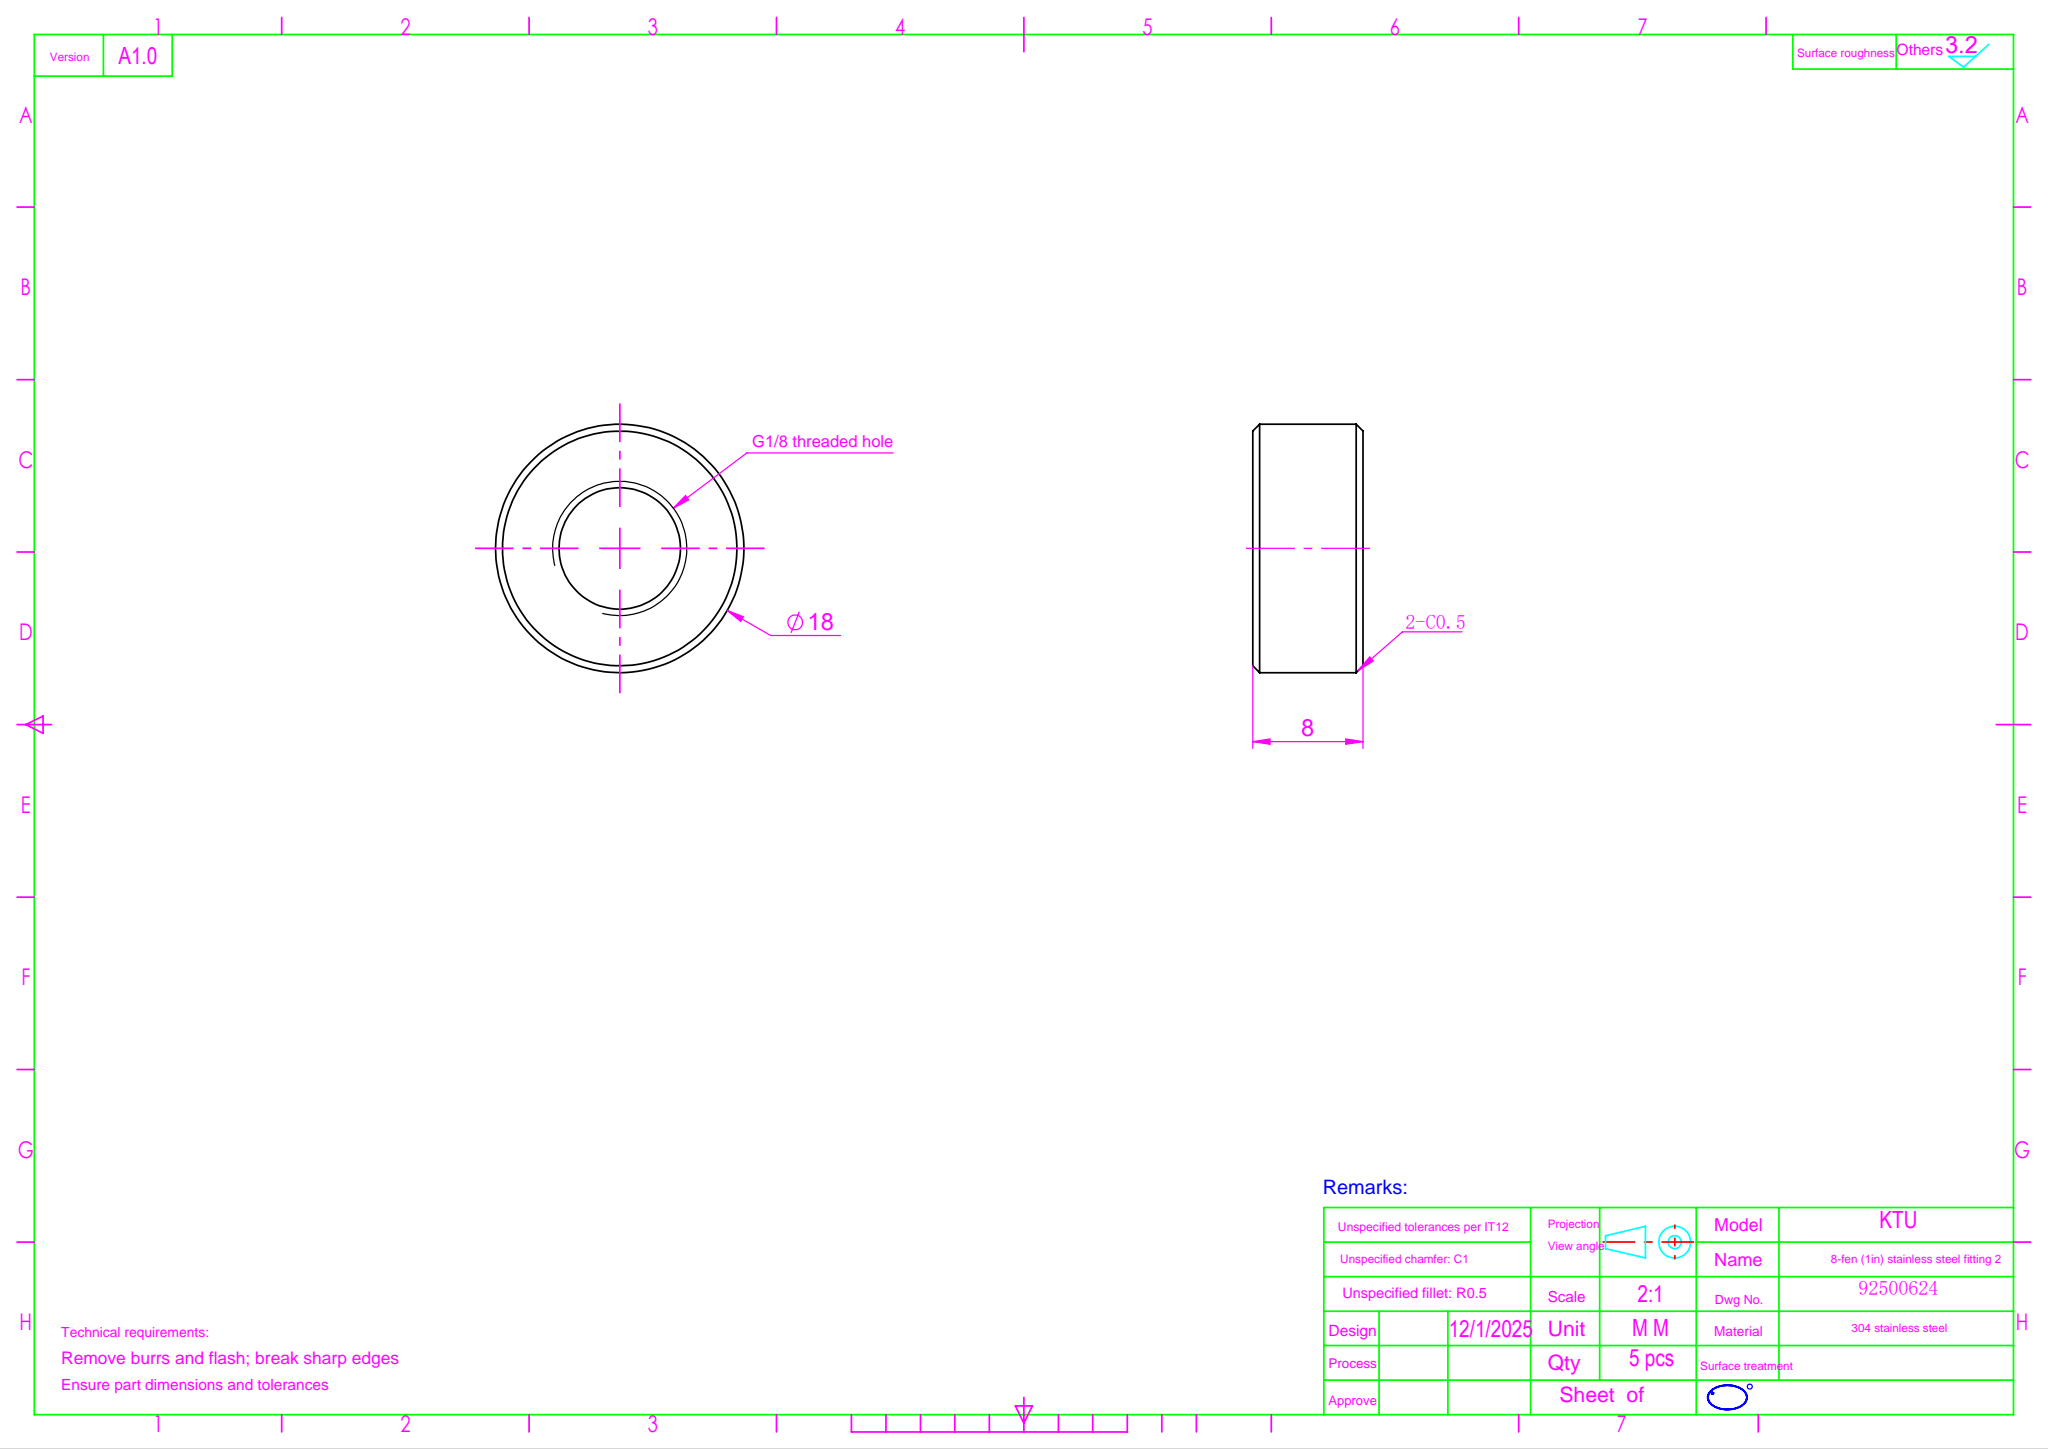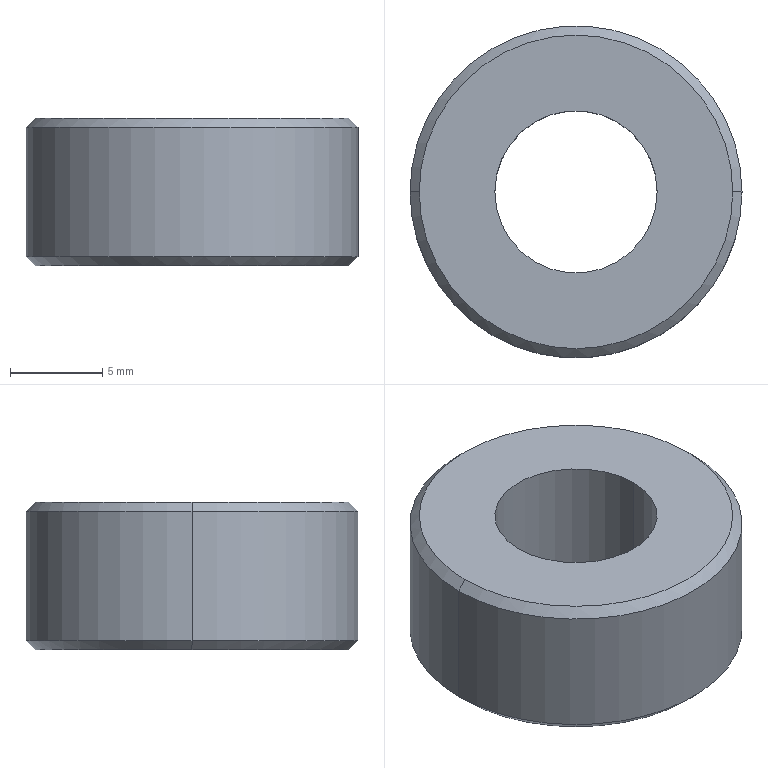Part | SolidWorks | features Chamfer 1, Extrusion 1, HoleWzd 1 | 1 solid | 10 faces | box 18 x 18 x 8 mm | volume 1535 mm3 | cone 4 | cylinder 4 | plane 2 | commonest cylinder face diameters 8.8 x2 18 x2
STEP:
#1=CARTESIAN_POINT('',(8.5,0.,8.));
#2=VERTEX_POINT('',#1);
#3=CARTESIAN_POINT('',(-8.5,0.,8.));
#4=VERTEX_POINT('',#3);
#5=CARTESIAN_POINT('',(0.,0.,8.));
#6=DIRECTION('',(0.,0.,1.));
#7=DIRECTION('',(1.,0.,0.));
#8=AXIS2_PLACEMENT_3D('',#5,#6,#7);
#9=CIRCLE('',#8,8.5);
#10=EDGE_CURVE('',#2,#4,#9,.T.);
#11=ORIENTED_EDGE('',*,*,#10,.F.);
#12=CARTESIAN_POINT('',(9.,0.,7.5));
#13=VERTEX_POINT('',#12);
#14=CARTESIAN_POINT('',(8.5,0.,8.));
#15=DIRECTION('',(0.7071,0.,-0.7071));
#16=VECTOR('',#15,1000.);
#17=LINE('',#14,#16);
#18=EDGE_CURVE('',#2,#13,#17,.T.);
#19=ORIENTED_EDGE('',*,*,#18,.T.);
#20=CARTESIAN_POINT('',(-9.,0.,7.5));
#21=VERTEX_POINT('',#20);
#22=CARTESIAN_POINT('',(0.,0.,7.5));
#23=DIRECTION('',(0.,0.,-1.));
#24=DIRECTION('',(1.,0.,0.));
#25=AXIS2_PLACEMENT_3D('',#22,#23,#24);
#26=CIRCLE('',#25,9.);
#27=EDGE_CURVE('',#21,#13,#26,.T.);
#28=ORIENTED_EDGE('',*,*,#27,.F.);
#29=CARTESIAN_POINT('',(-8.5,0.,8.));
#30=DIRECTION('',(-0.7071,0.,-0.7071));
#31=VECTOR('',#30,1000.);
#32=LINE('',#29,#31);
#33=EDGE_CURVE('',#4,#21,#32,.T.);
#34=ORIENTED_EDGE('',*,*,#33,.F.);
#35=EDGE_LOOP('',(#11,#19,#28,#34));
#36=FACE_OUTER_BOUND('',#35,.T.);
#37=CARTESIAN_POINT('',(0.,0.,8.));
#38=DIRECTION('',(0.,0.,-1.));
#39=DIRECTION('',(-1.,0.,0.));
#40=AXIS2_PLACEMENT_3D('',#37,#38,#39);
#41=CONICAL_SURFACE('',#40,8.5,0.7854);
#42=ADVANCED_FACE('',(#36),#41,.T.);
#43=CARTESIAN_POINT('',(-8.5,0.,0.));
#44=VERTEX_POINT('',#43);
#45=CARTESIAN_POINT('',(8.5,0.,0.));
#46=VERTEX_POINT('',#45);
#47=CARTESIAN_POINT('',(0.,0.,0.));
#48=DIRECTION('',(0.,0.,-1.));
#49=DIRECTION('',(1.,0.,0.));
#50=AXIS2_PLACEMENT_3D('',#47,#48,#49);
#51=CIRCLE('',#50,8.5);
#52=EDGE_CURVE('',#44,#46,#51,.T.);
#53=ORIENTED_EDGE('',*,*,#52,.F.);
#54=CARTESIAN_POINT('',(-9.,0.,0.5));
#55=VERTEX_POINT('',#54);
#56=CARTESIAN_POINT('',(-9.,0.,0.5));
#57=DIRECTION('',(-0.7071,0.,0.7071));
#58=VECTOR('',#57,1000.);
#59=LINE('',#56,#58);
#60=EDGE_CURVE('',#44,#55,#59,.T.);
#61=ORIENTED_EDGE('',*,*,#60,.T.);
#62=CARTESIAN_POINT('',(9.,0.,0.5));
#63=VERTEX_POINT('',#62);
#64=CARTESIAN_POINT('',(0.,0.,0.5));
#65=DIRECTION('',(0.,0.,1.));
#66=DIRECTION('',(1.,0.,0.));
#67=AXIS2_PLACEMENT_3D('',#64,#65,#66);
#68=CIRCLE('',#67,9.);
#69=EDGE_CURVE('',#63,#55,#68,.T.);
#70=ORIENTED_EDGE('',*,*,#69,.F.);
#71=CARTESIAN_POINT('',(9.,0.,0.5));
#72=DIRECTION('',(0.7071,0.,0.7071));
#73=VECTOR('',#72,1000.);
#74=LINE('',#71,#73);
#75=EDGE_CURVE('',#46,#63,#74,.T.);
#76=ORIENTED_EDGE('',*,*,#75,.F.);
#77=EDGE_LOOP('',(#53,#61,#70,#76));
#78=FACE_OUTER_BOUND('',#77,.T.);
#79=CARTESIAN_POINT('',(0.,0.,0.5));
#80=DIRECTION('',(0.,0.,1.));
#81=DIRECTION('',(1.,0.,0.));
#82=AXIS2_PLACEMENT_3D('',#79,#80,#81);
#83=CONICAL_SURFACE('',#82,9.,0.7854);
#84=ADVANCED_FACE('',(#78),#83,.T.);
#85=CARTESIAN_POINT('',(-4.4,0.,0.));
#86=VERTEX_POINT('',#85);
#87=CARTESIAN_POINT('',(4.4,0.,0.));
#88=VERTEX_POINT('',#87);
#89=CARTESIAN_POINT('',(0.,0.,0.));
#90=DIRECTION('',(0.,0.,1.));
#91=DIRECTION('',(1.,0.,0.));
#92=AXIS2_PLACEMENT_3D('',#89,#90,#91);
#93=CIRCLE('',#92,4.4);
#94=EDGE_CURVE('',#86,#88,#93,.T.);
#95=ORIENTED_EDGE('',*,*,#94,.F.);
#96=CARTESIAN_POINT('',(-4.4,0.,8.));
#97=VERTEX_POINT('',#96);
#98=CARTESIAN_POINT('',(-4.4,0.,8.));
#99=DIRECTION('',(0.,0.,1.));
#100=VECTOR('',#99,1000.);
#101=LINE('',#98,#100);
#102=EDGE_CURVE('',#86,#97,#101,.T.);
#103=ORIENTED_EDGE('',*,*,#102,.T.);
#104=CARTESIAN_POINT('',(4.4,0.,8.));
#105=VERTEX_POINT('',#104);
#106=CARTESIAN_POINT('',(0.,0.,8.));
#107=DIRECTION('',(0.,0.,1.));
#108=DIRECTION('',(1.,0.,0.));
#109=AXIS2_PLACEMENT_3D('',#106,#107,#108);
#110=CIRCLE('',#109,4.4);
#111=EDGE_CURVE('',#97,#105,#110,.T.);
#112=ORIENTED_EDGE('',*,*,#111,.T.);
#113=CARTESIAN_POINT('',(4.4,0.,8.));
#114=DIRECTION('',(0.,0.,1.));
#115=VECTOR('',#114,1000.);
#116=LINE('',#113,#115);
#117=EDGE_CURVE('',#88,#105,#116,.T.);
#118=ORIENTED_EDGE('',*,*,#117,.F.);
#119=EDGE_LOOP('',(#95,#103,#112,#118));
#120=FACE_OUTER_BOUND('',#119,.T.);
#121=CARTESIAN_POINT('',(0.,0.,8.));
#122=DIRECTION('',(0.,0.,1.));
#123=DIRECTION('',(1.,0.,0.));
#124=AXIS2_PLACEMENT_3D('',#121,#122,#123);
#125=CYLINDRICAL_SURFACE('',#124,4.4);
#126=ADVANCED_FACE('',(#120),#125,.F.);
#127=ORIENTED_EDGE('',*,*,#27,.T.);
#128=CARTESIAN_POINT('',(9.,0.,8.));
#129=DIRECTION('',(0.,0.,-1.));
#130=VECTOR('',#129,1000.);
#131=LINE('',#128,#130);
#132=EDGE_CURVE('',#13,#63,#131,.T.);
#133=ORIENTED_EDGE('',*,*,#132,.T.);
#134=ORIENTED_EDGE('',*,*,#69,.T.);
#135=CARTESIAN_POINT('',(-9.,0.,8.));
#136=DIRECTION('',(0.,0.,-1.));
#137=VECTOR('',#136,1000.);
#138=LINE('',#135,#137);
#139=EDGE_CURVE('',#21,#55,#138,.T.);
#140=ORIENTED_EDGE('',*,*,#139,.F.);
#141=EDGE_LOOP('',(#127,#133,#134,#140));
#142=FACE_OUTER_BOUND('',#141,.T.);
#143=CARTESIAN_POINT('',(0.,0.,8.));
#144=DIRECTION('',(0.,0.,-1.));
#145=DIRECTION('',(-1.,0.,0.));
#146=AXIS2_PLACEMENT_3D('',#143,#144,#145);
#147=CYLINDRICAL_SURFACE('',#146,9.);
#148=ADVANCED_FACE('',(#142),#147,.T.);
#149=ORIENTED_EDGE('',*,*,#132,.F.);
#150=CARTESIAN_POINT('',(0.,0.,7.5));
#151=DIRECTION('',(0.,0.,-1.));
#152=DIRECTION('',(1.,0.,0.));
#153=AXIS2_PLACEMENT_3D('',#150,#151,#152);
#154=CIRCLE('',#153,9.);
#155=EDGE_CURVE('',#13,#21,#154,.T.);
#156=ORIENTED_EDGE('',*,*,#155,.T.);
#157=ORIENTED_EDGE('',*,*,#139,.T.);
#158=CARTESIAN_POINT('',(0.,0.,0.5));
#159=DIRECTION('',(0.,0.,1.));
#160=DIRECTION('',(1.,0.,0.));
#161=AXIS2_PLACEMENT_3D('',#158,#159,#160);
#162=CIRCLE('',#161,9.);
#163=EDGE_CURVE('',#55,#63,#162,.T.);
#164=ORIENTED_EDGE('',*,*,#163,.T.);
#165=EDGE_LOOP('',(#149,#156,#157,#164));
#166=FACE_OUTER_BOUND('',#165,.T.);
#167=CARTESIAN_POINT('',(0.,0.,8.));
#168=DIRECTION('',(0.,0.,-1.));
#169=DIRECTION('',(-1.,0.,0.));
#170=AXIS2_PLACEMENT_3D('',#167,#168,#169);
#171=CYLINDRICAL_SURFACE('',#170,9.);
#172=ADVANCED_FACE('',(#166),#171,.T.);
#173=CARTESIAN_POINT('',(0.,0.,8.));
#174=DIRECTION('',(0.,0.,1.));
#175=DIRECTION('',(1.,0.,0.));
#176=AXIS2_PLACEMENT_3D('',#173,#174,#175);
#177=CIRCLE('',#176,8.5);
#178=EDGE_CURVE('',#4,#2,#177,.T.);
#179=ORIENTED_EDGE('',*,*,#178,.T.);
#180=ORIENTED_EDGE('',*,*,#10,.T.);
#181=EDGE_LOOP('',(#179,#180));
#182=FACE_OUTER_BOUND('',#181,.T.);
#183=CARTESIAN_POINT('',(0.,0.,8.));
#184=DIRECTION('',(0.,0.,1.));
#185=DIRECTION('',(1.,0.,0.));
#186=AXIS2_PLACEMENT_3D('',#183,#184,#185);
#187=CIRCLE('',#186,4.4);
#188=EDGE_CURVE('',#105,#97,#187,.T.);
#189=ORIENTED_EDGE('',*,*,#188,.F.);
#190=ORIENTED_EDGE('',*,*,#111,.F.);
#191=EDGE_LOOP('',(#189,#190));
#192=FACE_BOUND('',#191,.T.);
#193=CARTESIAN_POINT('',(0.,0.,8.));
#194=DIRECTION('',(0.,0.,1.));
#195=DIRECTION('',(1.,0.,0.));
#196=AXIS2_PLACEMENT_3D('',#193,#194,#195);
#197=PLANE('',#196);
#198=ADVANCED_FACE('',(#182,#192),#197,.T.);
#199=CARTESIAN_POINT('',(0.,0.,0.));
#200=DIRECTION('',(0.,0.,-1.));
#201=DIRECTION('',(1.,0.,0.));
#202=AXIS2_PLACEMENT_3D('',#199,#200,#201);
#203=CIRCLE('',#202,8.5);
#204=EDGE_CURVE('',#46,#44,#203,.T.);
#205=ORIENTED_EDGE('',*,*,#204,.T.);
#206=ORIENTED_EDGE('',*,*,#52,.T.);
#207=EDGE_LOOP('',(#205,#206));
#208=FACE_OUTER_BOUND('',#207,.T.);
#209=CARTESIAN_POINT('',(0.,0.,0.));
#210=DIRECTION('',(0.,0.,1.));
#211=DIRECTION('',(1.,0.,0.));
#212=AXIS2_PLACEMENT_3D('',#209,#210,#211);
#213=CIRCLE('',#212,4.4);
#214=EDGE_CURVE('',#88,#86,#213,.T.);
#215=ORIENTED_EDGE('',*,*,#214,.T.);
#216=ORIENTED_EDGE('',*,*,#94,.T.);
#217=EDGE_LOOP('',(#215,#216));
#218=FACE_BOUND('',#217,.T.);
#219=CARTESIAN_POINT('',(0.,0.,0.));
#220=DIRECTION('',(0.,0.,1.));
#221=DIRECTION('',(1.,0.,0.));
#222=AXIS2_PLACEMENT_3D('',#219,#220,#221);
#223=PLANE('',#222);
#224=ADVANCED_FACE('',(#208,#218),#223,.F.);
#225=ORIENTED_EDGE('',*,*,#102,.F.);
#226=ORIENTED_EDGE('',*,*,#214,.F.);
#227=ORIENTED_EDGE('',*,*,#117,.T.);
#228=ORIENTED_EDGE('',*,*,#188,.T.);
#229=EDGE_LOOP('',(#225,#226,#227,#228));
#230=FACE_OUTER_BOUND('',#229,.T.);
#231=CARTESIAN_POINT('',(0.,0.,8.));
#232=DIRECTION('',(0.,0.,1.));
#233=DIRECTION('',(1.,0.,0.));
#234=AXIS2_PLACEMENT_3D('',#231,#232,#233);
#235=CYLINDRICAL_SURFACE('',#234,4.4);
#236=ADVANCED_FACE('',(#230),#235,.F.);
#237=ORIENTED_EDGE('',*,*,#60,.F.);
#238=ORIENTED_EDGE('',*,*,#204,.F.);
#239=ORIENTED_EDGE('',*,*,#75,.T.);
#240=ORIENTED_EDGE('',*,*,#163,.F.);
#241=EDGE_LOOP('',(#237,#238,#239,#240));
#242=FACE_OUTER_BOUND('',#241,.T.);
#243=CARTESIAN_POINT('',(0.,0.,0.5));
#244=DIRECTION('',(0.,0.,1.));
#245=DIRECTION('',(1.,0.,0.));
#246=AXIS2_PLACEMENT_3D('',#243,#244,#245);
#247=CONICAL_SURFACE('',#246,9.,0.7854);
#248=ADVANCED_FACE('',(#242),#247,.T.);
#249=ORIENTED_EDGE('',*,*,#18,.F.);
#250=ORIENTED_EDGE('',*,*,#178,.F.);
#251=ORIENTED_EDGE('',*,*,#33,.T.);
#252=ORIENTED_EDGE('',*,*,#155,.F.);
#253=EDGE_LOOP('',(#249,#250,#251,#252));
#254=FACE_OUTER_BOUND('',#253,.T.);
#255=CARTESIAN_POINT('',(0.,0.,8.));
#256=DIRECTION('',(0.,0.,-1.));
#257=DIRECTION('',(-1.,0.,0.));
#258=AXIS2_PLACEMENT_3D('',#255,#256,#257);
#259=CONICAL_SURFACE('',#258,8.5,0.7854);
#260=ADVANCED_FACE('',(#254),#259,.T.);
#261=CLOSED_SHELL('',(#42,#84,#126,#148,#172,#198,#224,#236,#248,#260));
#262=MANIFOLD_SOLID_BREP('',#261);
#263=CARTESIAN_POINT('',(0.,0.,0.));
#264=DIRECTION('',(0.,0.,1.));
#265=DIRECTION('',(1.,0.,0.));
#266=AXIS2_PLACEMENT_3D('',#263,#264,#265);
#267=(LENGTH_UNIT()NAMED_UNIT(*)SI_UNIT(.MILLI.,.METRE.));
#268=UNCERTAINTY_MEASURE_WITH_UNIT(LENGTH_MEASURE(0.00001),#267,'','');
#269=(NAMED_UNIT(*)PLANE_ANGLE_UNIT()SI_UNIT($,.RADIAN.));
#270=(NAMED_UNIT(*)SI_UNIT($,.STERADIAN.)SOLID_ANGLE_UNIT());
#271=(GEOMETRIC_REPRESENTATION_CONTEXT(3)GLOBAL_UNCERTAINTY_ASSIGNED_CONTEXT((#268))GLOBAL_UNIT_ASSIGNED_CONTEXT((#267,#269,#270))REPRESENTATION_CONTEXT('',''));
#272=ADVANCED_BREP_SHAPE_REPRESENTATION('',(#262,#266),#271);